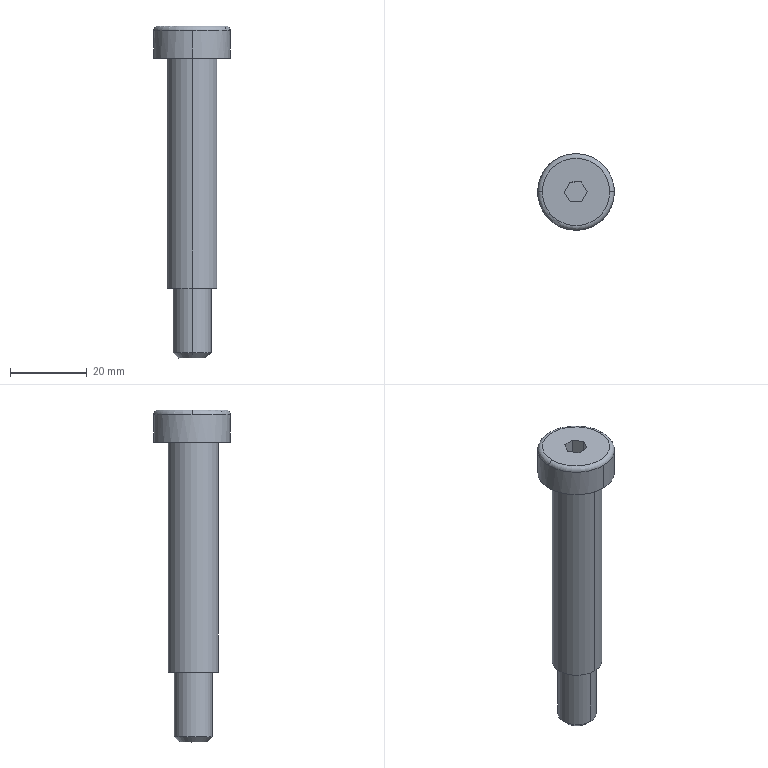Part | SolidWorks | features BaseBody 1 | 1 solid | 21 faces | box 20.001 x 20 x 86.624 mm | volume 11847 mm3 | plane 11 | cylinder 6 | torus 2 | cone 2 | commonest cylinder face diameters 10 x2 13 x2 20 x2
STEP:
#1=CARTESIAN_POINT('',(405.875,-5.722,120.785));
#2=VERTEX_POINT('',#1);
#3=CARTESIAN_POINT('',(396.085,-15.72,120.784));
#4=VERTEX_POINT('',#3);
#5=CARTESIAN_POINT('',(406.085,-15.72,120.785));
#6=DIRECTION('',(-0.0001435,-0.000000521,1.));
#7=DIRECTION('',(0.02104,-0.9998,0.000002497));
#8=AXIS2_PLACEMENT_3D('',#5,#6,#7);
#9=CIRCLE('',#8,10.);
#10=EDGE_CURVE('',#2,#4,#9,.T.);
#11=ORIENTED_EDGE('',*,*,#10,.T.);
#12=CARTESIAN_POINT('',(397.285,-15.72,121.984));
#13=VERTEX_POINT('',#12);
#14=CARTESIAN_POINT('',(397.285,-15.72,120.784));
#15=DIRECTION('',(0.,1.,0.000000521));
#16=DIRECTION('',(0.,-0.000000521,1.));
#17=AXIS2_PLACEMENT_3D('',#14,#15,#16);
#18=CIRCLE('',#17,1.2);
#19=EDGE_CURVE('',#4,#13,#18,.T.);
#20=ORIENTED_EDGE('',*,*,#19,.T.);
#21=CARTESIAN_POINT('',(414.885,-15.72,121.986));
#22=VERTEX_POINT('',#21);
#23=CARTESIAN_POINT('',(406.085,-15.72,121.985));
#24=DIRECTION('',(-0.0001435,-0.000000521,1.));
#25=DIRECTION('',(-1.,0.,-0.0001435));
#26=AXIS2_PLACEMENT_3D('',#23,#24,#25);
#27=CIRCLE('',#26,8.8);
#28=EDGE_CURVE('',#22,#13,#27,.T.);
#29=ORIENTED_EDGE('',*,*,#28,.F.);
#30=CARTESIAN_POINT('',(416.085,-15.72,120.786));
#31=VERTEX_POINT('',#30);
#32=CARTESIAN_POINT('',(414.885,-15.72,120.786));
#33=DIRECTION('',(0.,-1.,-0.000000521));
#34=DIRECTION('',(0.,0.000000521,-1.));
#35=AXIS2_PLACEMENT_3D('',#32,#33,#34);
#36=CIRCLE('',#35,1.2);
#37=EDGE_CURVE('',#31,#22,#36,.T.);
#38=ORIENTED_EDGE('',*,*,#37,.F.);
#39=CARTESIAN_POINT('',(406.085,-15.72,120.785));
#40=DIRECTION('',(-0.0001435,-0.000000521,1.));
#41=DIRECTION('',(0.02104,-0.9998,0.000002497));
#42=AXIS2_PLACEMENT_3D('',#39,#40,#41);
#43=CIRCLE('',#42,10.);
#44=EDGE_CURVE('',#31,#2,#43,.T.);
#45=ORIENTED_EDGE('',*,*,#44,.T.);
#46=EDGE_LOOP('',(#11,#20,#29,#38,#45));
#47=FACE_OUTER_BOUND('',#46,.T.);
#48=CARTESIAN_POINT('',(406.085,-15.72,120.785));
#49=DIRECTION('',(-0.0001435,-0.000000521,1.));
#50=DIRECTION('',(1.,0.,0.0001435));
#51=AXIS2_PLACEMENT_3D('',#48,#49,#50);
#52=TOROIDAL_SURFACE('',#51,8.8,1.2);
#53=ADVANCED_FACE('',(#47),#52,.T.);
#54=CARTESIAN_POINT('',(406.296,-25.717,113.585));
#55=VERTEX_POINT('',#54);
#56=CARTESIAN_POINT('',(405.876,-5.722,113.585));
#57=VERTEX_POINT('',#56);
#58=CARTESIAN_POINT('',(406.086,-15.72,113.585));
#59=DIRECTION('',(0.0001435,0.000000521,-1.));
#60=DIRECTION('',(-1.,0.,-0.0001435));
#61=AXIS2_PLACEMENT_3D('',#58,#59,#60);
#62=CIRCLE('',#61,10.);
#63=EDGE_CURVE('',#55,#57,#62,.T.);
#64=ORIENTED_EDGE('',*,*,#63,.F.);
#65=CARTESIAN_POINT('',(406.295,-25.717,120.785));
#66=VERTEX_POINT('',#65);
#67=CARTESIAN_POINT('',(406.296,-25.717,113.585));
#68=DIRECTION('',(-0.0001435,-0.000000521,1.));
#69=VECTOR('',#68,1000.);
#70=LINE('',#67,#69);
#71=EDGE_CURVE('',#55,#66,#70,.T.);
#72=ORIENTED_EDGE('',*,*,#71,.T.);
#73=CARTESIAN_POINT('',(406.085,-15.72,120.785));
#74=DIRECTION('',(-0.0001435,-0.000000521,1.));
#75=DIRECTION('',(0.02104,-0.9998,0.000002497));
#76=AXIS2_PLACEMENT_3D('',#73,#74,#75);
#77=CIRCLE('',#76,10.);
#78=EDGE_CURVE('',#4,#66,#77,.T.);
#79=ORIENTED_EDGE('',*,*,#78,.F.);
#80=ORIENTED_EDGE('',*,*,#10,.F.);
#81=CARTESIAN_POINT('',(405.876,-5.722,113.585));
#82=DIRECTION('',(-0.0001435,-0.000000521,1.));
#83=VECTOR('',#82,1000.);
#84=LINE('',#81,#83);
#85=EDGE_CURVE('',#57,#2,#84,.T.);
#86=ORIENTED_EDGE('',*,*,#85,.F.);
#87=EDGE_LOOP('',(#64,#72,#79,#80,#86));
#88=FACE_OUTER_BOUND('',#87,.T.);
#89=CARTESIAN_POINT('',(406.086,-15.72,113.585));
#90=DIRECTION('',(-0.0001435,-0.000000521,1.));
#91=DIRECTION('',(-0.02104,0.9998,-0.000002497));
#92=AXIS2_PLACEMENT_3D('',#89,#90,#91);
#93=CYLINDRICAL_SURFACE('',#92,10.);
#94=ADVANCED_FACE('',(#88),#93,.T.);
#95=CARTESIAN_POINT('',(405.959,-9.559,113.585));
#96=VERTEX_POINT('',#95);
#97=CARTESIAN_POINT('',(406.233,-22.556,113.585));
#98=VERTEX_POINT('',#97);
#99=CARTESIAN_POINT('',(406.096,-16.057,113.585));
#100=DIRECTION('',(-0.0001435,-0.000000521,1.));
#101=DIRECTION('',(0.02104,-0.9998,0.000002497));
#102=AXIS2_PLACEMENT_3D('',#99,#100,#101);
#103=CIRCLE('',#102,6.5);
#104=EDGE_CURVE('',#96,#98,#103,.T.);
#105=ORIENTED_EDGE('',*,*,#104,.F.);
#106=CARTESIAN_POINT('',(405.968,-9.558,53.585));
#107=VERTEX_POINT('',#106);
#108=CARTESIAN_POINT('',(405.964,-9.559,81.389));
#109=DIRECTION('',(0.0001435,0.000000521,-1.));
#110=VECTOR('',#109,1000.);
#111=LINE('',#108,#110);
#112=EDGE_CURVE('',#96,#107,#111,.T.);
#113=ORIENTED_EDGE('',*,*,#112,.T.);
#114=CARTESIAN_POINT('',(406.242,-22.556,53.585));
#115=VERTEX_POINT('',#114);
#116=CARTESIAN_POINT('',(406.105,-16.057,53.585));
#117=DIRECTION('',(0.0001435,0.000000521,-1.));
#118=DIRECTION('',(-1.,0.,-0.0001435));
#119=AXIS2_PLACEMENT_3D('',#116,#117,#118);
#120=CIRCLE('',#119,6.5);
#121=EDGE_CURVE('',#115,#107,#120,.T.);
#122=ORIENTED_EDGE('',*,*,#121,.F.);
#123=CARTESIAN_POINT('',(406.238,-22.556,81.389));
#124=DIRECTION('',(0.0001435,0.000000521,-1.));
#125=VECTOR('',#124,1000.);
#126=LINE('',#123,#125);
#127=EDGE_CURVE('',#98,#115,#126,.T.);
#128=ORIENTED_EDGE('',*,*,#127,.F.);
#129=EDGE_LOOP('',(#105,#113,#122,#128));
#130=FACE_OUTER_BOUND('',#129,.T.);
#131=CARTESIAN_POINT('',(406.101,-16.057,81.389));
#132=DIRECTION('',(0.0001435,0.000000521,-1.));
#133=DIRECTION('',(0.02104,-0.9998,0.000002497));
#134=AXIS2_PLACEMENT_3D('',#131,#132,#133);
#135=CYLINDRICAL_SURFACE('',#134,6.5);
#136=ADVANCED_FACE('',(#130),#135,.T.);
#137=CARTESIAN_POINT('',(405.998,-11.058,53.585));
#138=VERTEX_POINT('',#137);
#139=CARTESIAN_POINT('',(406.208,-21.056,53.585));
#140=VERTEX_POINT('',#139);
#141=CARTESIAN_POINT('',(406.103,-16.057,53.585));
#142=DIRECTION('',(-0.0001435,-0.000000521,1.));
#143=DIRECTION('',(0.02104,-0.9998,0.000002497));
#144=AXIS2_PLACEMENT_3D('',#141,#142,#143);
#145=CIRCLE('',#144,5.);
#146=EDGE_CURVE('',#138,#140,#145,.T.);
#147=ORIENTED_EDGE('',*,*,#146,.F.);
#148=CARTESIAN_POINT('',(406.,-11.058,36.763));
#149=VERTEX_POINT('',#148);
#150=CARTESIAN_POINT('',(405.999,-11.058,48.803));
#151=DIRECTION('',(0.0001435,0.000000521,-1.));
#152=VECTOR('',#151,1000.);
#153=LINE('',#150,#152);
#154=EDGE_CURVE('',#138,#149,#153,.T.);
#155=ORIENTED_EDGE('',*,*,#154,.T.);
#156=CARTESIAN_POINT('',(406.211,-21.056,36.763));
#157=VERTEX_POINT('',#156);
#158=CARTESIAN_POINT('',(406.106,-16.057,36.763));
#159=DIRECTION('',(0.0001435,0.000000521,-1.));
#160=DIRECTION('',(0.02104,-0.9998,0.000002497));
#161=AXIS2_PLACEMENT_3D('',#158,#159,#160);
#162=CIRCLE('',#161,5.);
#163=EDGE_CURVE('',#157,#149,#162,.T.);
#164=ORIENTED_EDGE('',*,*,#163,.F.);
#165=CARTESIAN_POINT('',(406.209,-21.056,48.803));
#166=DIRECTION('',(0.0001435,0.000000521,-1.));
#167=VECTOR('',#166,1000.);
#168=LINE('',#165,#167);
#169=EDGE_CURVE('',#140,#157,#168,.T.);
#170=ORIENTED_EDGE('',*,*,#169,.F.);
#171=EDGE_LOOP('',(#147,#155,#164,#170));
#172=FACE_OUTER_BOUND('',#171,.T.);
#173=CARTESIAN_POINT('',(406.104,-16.057,48.803));
#174=DIRECTION('',(0.0001435,0.000000521,-1.));
#175=DIRECTION('',(0.02104,-0.9998,0.000002497));
#176=AXIS2_PLACEMENT_3D('',#173,#174,#175);
#177=CYLINDRICAL_SURFACE('',#176,5.);
#178=ADVANCED_FACE('',(#172),#177,.T.);
#179=CARTESIAN_POINT('',(406.181,-19.656,35.363));
#180=VERTEX_POINT('',#179);
#181=CARTESIAN_POINT('',(406.03,-12.458,35.363));
#182=VERTEX_POINT('',#181);
#183=CARTESIAN_POINT('',(406.106,-16.057,35.363));
#184=DIRECTION('',(0.0001435,0.000000521,-1.));
#185=DIRECTION('',(0.02104,-0.9998,0.000002497));
#186=AXIS2_PLACEMENT_3D('',#183,#184,#185);
#187=CIRCLE('',#186,3.6);
#188=EDGE_CURVE('',#180,#182,#187,.T.);
#189=ORIENTED_EDGE('',*,*,#188,.F.);
#190=CARTESIAN_POINT('',(406.196,-20.356,36.063));
#191=DIRECTION('',(0.01477,-0.707,0.7071));
#192=VECTOR('',#191,1000.);
#193=LINE('',#190,#192);
#194=EDGE_CURVE('',#180,#157,#193,.T.);
#195=ORIENTED_EDGE('',*,*,#194,.T.);
#196=ORIENTED_EDGE('',*,*,#163,.T.);
#197=CARTESIAN_POINT('',(406.015,-11.758,36.063));
#198=DIRECTION('',(-0.01498,0.7069,0.7071));
#199=VECTOR('',#198,1000.);
#200=LINE('',#197,#199);
#201=EDGE_CURVE('',#182,#149,#200,.T.);
#202=ORIENTED_EDGE('',*,*,#201,.F.);
#203=EDGE_LOOP('',(#189,#195,#196,#202));
#204=FACE_OUTER_BOUND('',#203,.T.);
#205=CARTESIAN_POINT('',(406.106,-16.057,36.063));
#206=DIRECTION('',(-0.0001435,-0.000000521,1.));
#207=DIRECTION('',(-0.02104,0.9998,-0.000002497));
#208=AXIS2_PLACEMENT_3D('',#205,#206,#207);
#209=CONICAL_SURFACE('',#208,4.3,0.7854);
#210=ADVANCED_FACE('',(#204),#209,.T.);
#211=CARTESIAN_POINT('',(406.106,-16.057,35.363));
#212=DIRECTION('',(0.0001435,0.000000521,-1.));
#213=DIRECTION('',(0.02104,-0.9998,0.000002497));
#214=AXIS2_PLACEMENT_3D('',#211,#212,#213);
#215=CIRCLE('',#214,3.6);
#216=EDGE_CURVE('',#182,#180,#215,.T.);
#217=ORIENTED_EDGE('',*,*,#216,.T.);
#218=ORIENTED_EDGE('',*,*,#188,.T.);
#219=EDGE_LOOP('',(#217,#218));
#220=FACE_OUTER_BOUND('',#219,.T.);
#221=CARTESIAN_POINT('',(406.106,-16.057,35.363));
#222=DIRECTION('',(0.0001435,0.000000521,-1.));
#223=DIRECTION('',(0.,-1.,-0.000000521));
#224=AXIS2_PLACEMENT_3D('',#221,#222,#223);
#225=PLANE('',#224);
#226=ADVANCED_FACE('',(#220),#225,.T.);
#227=ORIENTED_EDGE('',*,*,#194,.F.);
#228=ORIENTED_EDGE('',*,*,#216,.F.);
#229=ORIENTED_EDGE('',*,*,#201,.T.);
#230=CARTESIAN_POINT('',(406.106,-16.057,36.763));
#231=DIRECTION('',(0.0001435,0.000000521,-1.));
#232=DIRECTION('',(0.02104,-0.9998,0.000002497));
#233=AXIS2_PLACEMENT_3D('',#230,#231,#232);
#234=CIRCLE('',#233,5.);
#235=EDGE_CURVE('',#149,#157,#234,.T.);
#236=ORIENTED_EDGE('',*,*,#235,.T.);
#237=EDGE_LOOP('',(#227,#228,#229,#236));
#238=FACE_OUTER_BOUND('',#237,.T.);
#239=CARTESIAN_POINT('',(406.106,-16.057,36.063));
#240=DIRECTION('',(-0.0001435,-0.000000521,1.));
#241=DIRECTION('',(-0.02104,0.9998,-0.000002497));
#242=AXIS2_PLACEMENT_3D('',#239,#240,#241);
#243=CONICAL_SURFACE('',#242,4.3,0.7854);
#244=ADVANCED_FACE('',(#238),#243,.T.);
#245=ORIENTED_EDGE('',*,*,#154,.F.);
#246=CARTESIAN_POINT('',(406.103,-16.057,53.585));
#247=DIRECTION('',(-0.0001435,-0.000000521,1.));
#248=DIRECTION('',(0.02104,-0.9998,0.000002497));
#249=AXIS2_PLACEMENT_3D('',#246,#247,#248);
#250=CIRCLE('',#249,5.);
#251=EDGE_CURVE('',#140,#138,#250,.T.);
#252=ORIENTED_EDGE('',*,*,#251,.F.);
#253=ORIENTED_EDGE('',*,*,#169,.T.);
#254=ORIENTED_EDGE('',*,*,#235,.F.);
#255=EDGE_LOOP('',(#245,#252,#253,#254));
#256=FACE_OUTER_BOUND('',#255,.T.);
#257=CARTESIAN_POINT('',(406.104,-16.057,48.803));
#258=DIRECTION('',(0.0001435,0.000000521,-1.));
#259=DIRECTION('',(0.02104,-0.9998,0.000002497));
#260=AXIS2_PLACEMENT_3D('',#257,#258,#259);
#261=CYLINDRICAL_SURFACE('',#260,5.);
#262=ADVANCED_FACE('',(#256),#261,.T.);
#263=ORIENTED_EDGE('',*,*,#251,.T.);
#264=ORIENTED_EDGE('',*,*,#146,.T.);
#265=EDGE_LOOP('',(#263,#264));
#266=FACE_BOUND('',#265,.T.);
#267=ORIENTED_EDGE('',*,*,#121,.T.);
#268=CARTESIAN_POINT('',(406.105,-16.057,53.585));
#269=DIRECTION('',(0.0001435,0.000000521,-1.));
#270=DIRECTION('',(-1.,0.,-0.0001435));
#271=AXIS2_PLACEMENT_3D('',#268,#269,#270);
#272=CIRCLE('',#271,6.5);
#273=EDGE_CURVE('',#107,#115,#272,.T.);
#274=ORIENTED_EDGE('',*,*,#273,.T.);
#275=EDGE_LOOP('',(#267,#274));
#276=FACE_OUTER_BOUND('',#275,.T.);
#277=CARTESIAN_POINT('',(406.09,-15.72,53.585));
#278=DIRECTION('',(0.0001435,0.000000521,-1.));
#279=DIRECTION('',(0.,-1.,-0.000000521));
#280=AXIS2_PLACEMENT_3D('',#277,#278,#279);
#281=PLANE('',#280);
#282=ADVANCED_FACE('',(#266,#276),#281,.T.);
#283=ORIENTED_EDGE('',*,*,#112,.F.);
#284=CARTESIAN_POINT('',(406.096,-16.057,113.585));
#285=DIRECTION('',(-0.0001435,-0.000000521,1.));
#286=DIRECTION('',(0.02104,-0.9998,0.000002497));
#287=AXIS2_PLACEMENT_3D('',#284,#285,#286);
#288=CIRCLE('',#287,6.5);
#289=EDGE_CURVE('',#98,#96,#288,.T.);
#290=ORIENTED_EDGE('',*,*,#289,.F.);
#291=ORIENTED_EDGE('',*,*,#127,.T.);
#292=ORIENTED_EDGE('',*,*,#273,.F.);
#293=EDGE_LOOP('',(#283,#290,#291,#292));
#294=FACE_OUTER_BOUND('',#293,.T.);
#295=CARTESIAN_POINT('',(406.101,-16.057,81.389));
#296=DIRECTION('',(0.0001435,0.000000521,-1.));
#297=DIRECTION('',(0.02104,-0.9998,0.000002497));
#298=AXIS2_PLACEMENT_3D('',#295,#296,#297);
#299=CYLINDRICAL_SURFACE('',#298,6.5);
#300=ADVANCED_FACE('',(#294),#299,.T.);
#301=ORIENTED_EDGE('',*,*,#289,.T.);
#302=ORIENTED_EDGE('',*,*,#104,.T.);
#303=EDGE_LOOP('',(#301,#302));
#304=FACE_BOUND('',#303,.T.);
#305=CARTESIAN_POINT('',(406.086,-15.72,113.585));
#306=DIRECTION('',(0.0001435,0.000000521,-1.));
#307=DIRECTION('',(-1.,0.,-0.0001435));
#308=AXIS2_PLACEMENT_3D('',#305,#306,#307);
#309=CIRCLE('',#308,10.);
#310=EDGE_CURVE('',#57,#55,#309,.T.);
#311=ORIENTED_EDGE('',*,*,#310,.T.);
#312=ORIENTED_EDGE('',*,*,#63,.T.);
#313=EDGE_LOOP('',(#311,#312));
#314=FACE_OUTER_BOUND('',#313,.T.);
#315=CARTESIAN_POINT('',(406.086,-15.72,113.585));
#316=DIRECTION('',(0.0001435,0.000000521,-1.));
#317=DIRECTION('',(0.,-1.,-0.000000521));
#318=AXIS2_PLACEMENT_3D('',#315,#316,#317);
#319=PLANE('',#318);
#320=ADVANCED_FACE('',(#304,#314),#319,.T.);
#321=ORIENTED_EDGE('',*,*,#71,.F.);
#322=ORIENTED_EDGE('',*,*,#310,.F.);
#323=ORIENTED_EDGE('',*,*,#85,.T.);
#324=ORIENTED_EDGE('',*,*,#44,.F.);
#325=CARTESIAN_POINT('',(406.085,-15.72,120.785));
#326=DIRECTION('',(-0.0001435,-0.000000521,1.));
#327=DIRECTION('',(0.02104,-0.9998,0.000002497));
#328=AXIS2_PLACEMENT_3D('',#325,#326,#327);
#329=CIRCLE('',#328,10.);
#330=EDGE_CURVE('',#66,#31,#329,.T.);
#331=ORIENTED_EDGE('',*,*,#330,.F.);
#332=EDGE_LOOP('',(#321,#322,#323,#324,#331));
#333=FACE_OUTER_BOUND('',#332,.T.);
#334=CARTESIAN_POINT('',(406.086,-15.72,113.585));
#335=DIRECTION('',(-0.0001435,-0.000000521,1.));
#336=DIRECTION('',(-0.02104,0.9998,-0.000002497));
#337=AXIS2_PLACEMENT_3D('',#334,#335,#336);
#338=CYLINDRICAL_SURFACE('',#337,10.);
#339=ADVANCED_FACE('',(#333),#338,.T.);
#340=ORIENTED_EDGE('',*,*,#19,.F.);
#341=ORIENTED_EDGE('',*,*,#78,.T.);
#342=ORIENTED_EDGE('',*,*,#330,.T.);
#343=ORIENTED_EDGE('',*,*,#37,.T.);
#344=CARTESIAN_POINT('',(406.085,-15.72,121.985));
#345=DIRECTION('',(-0.0001435,-0.000000521,1.));
#346=DIRECTION('',(-1.,0.,-0.0001435));
#347=AXIS2_PLACEMENT_3D('',#344,#345,#346);
#348=CIRCLE('',#347,8.8);
#349=EDGE_CURVE('',#13,#22,#348,.T.);
#350=ORIENTED_EDGE('',*,*,#349,.F.);
#351=EDGE_LOOP('',(#340,#341,#342,#343,#350));
#352=FACE_OUTER_BOUND('',#351,.T.);
#353=CARTESIAN_POINT('',(406.085,-15.72,120.785));
#354=DIRECTION('',(-0.0001435,-0.000000521,1.));
#355=DIRECTION('',(1.,0.,0.0001435));
#356=AXIS2_PLACEMENT_3D('',#353,#354,#355);
#357=TOROIDAL_SURFACE('',#356,8.8,1.2);
#358=ADVANCED_FACE('',(#352),#357,.T.);
#359=CARTESIAN_POINT('',(404.584,-18.33,115.985));
#360=VERTEX_POINT('',#359);
#361=CARTESIAN_POINT('',(407.583,-18.267,115.985));
#362=VERTEX_POINT('',#361);
#363=CARTESIAN_POINT('',(404.584,-18.33,115.985));
#364=DIRECTION('',(0.9998,0.02104,0.0001435));
#365=VECTOR('',#364,1000.);
#366=LINE('',#363,#365);
#367=EDGE_CURVE('',#360,#362,#366,.T.);
#368=ORIENTED_EDGE('',*,*,#367,.T.);
#369=CARTESIAN_POINT('',(409.028,-15.638,115.985));
#370=VERTEX_POINT('',#369);
#371=CARTESIAN_POINT('',(407.583,-18.267,115.985));
#372=DIRECTION('',(0.4817,0.8764,0.00006956));
#373=VECTOR('',#372,1000.);
#374=LINE('',#371,#373);
#375=EDGE_CURVE('',#362,#370,#374,.T.);
#376=ORIENTED_EDGE('',*,*,#375,.T.);
#377=CARTESIAN_POINT('',(407.474,-13.072,115.985));
#378=VERTEX_POINT('',#377);
#379=CARTESIAN_POINT('',(409.028,-15.638,115.985));
#380=DIRECTION('',(-0.5181,0.8553,-0.00007389));
#381=VECTOR('',#380,1000.);
#382=LINE('',#379,#381);
#383=EDGE_CURVE('',#370,#378,#382,.T.);
#384=ORIENTED_EDGE('',*,*,#383,.T.);
#385=CARTESIAN_POINT('',(404.474,-13.135,115.985));
#386=VERTEX_POINT('',#385);
#387=CARTESIAN_POINT('',(407.474,-13.072,115.985));
#388=DIRECTION('',(-0.9998,-0.02104,-0.0001435));
#389=VECTOR('',#388,1000.);
#390=LINE('',#387,#389);
#391=EDGE_CURVE('',#378,#386,#390,.T.);
#392=ORIENTED_EDGE('',*,*,#391,.T.);
#393=CARTESIAN_POINT('',(403.029,-15.764,115.985));
#394=VERTEX_POINT('',#393);
#395=CARTESIAN_POINT('',(404.474,-13.135,115.985));
#396=DIRECTION('',(-0.4817,-0.8764,-0.00006956));
#397=VECTOR('',#396,1000.);
#398=LINE('',#395,#397);
#399=EDGE_CURVE('',#386,#394,#398,.T.);
#400=ORIENTED_EDGE('',*,*,#399,.T.);
#401=CARTESIAN_POINT('',(403.029,-15.764,115.985));
#402=DIRECTION('',(0.5181,-0.8553,0.00007389));
#403=VECTOR('',#402,1000.);
#404=LINE('',#401,#403);
#405=EDGE_CURVE('',#394,#360,#404,.T.);
#406=ORIENTED_EDGE('',*,*,#405,.T.);
#407=EDGE_LOOP('',(#368,#376,#384,#392,#400,#406));
#408=FACE_OUTER_BOUND('',#407,.T.);
#409=CARTESIAN_POINT('',(405.473,13.374,115.985));
#410=DIRECTION('',(-0.0001435,-0.000000521,1.));
#411=DIRECTION('',(-0.003633,1.,0.));
#412=AXIS2_PLACEMENT_3D('',#409,#410,#411);
#413=PLANE('',#412);
#414=ADVANCED_FACE('',(#408),#413,.T.);
#415=CARTESIAN_POINT('',(407.582,-18.267,121.985));
#416=VERTEX_POINT('',#415);
#417=CARTESIAN_POINT('',(407.582,-18.267,121.985));
#418=DIRECTION('',(0.0001435,0.000000521,-1.));
#419=VECTOR('',#418,1000.);
#420=LINE('',#417,#419);
#421=EDGE_CURVE('',#416,#362,#420,.T.);
#422=ORIENTED_EDGE('',*,*,#421,.T.);
#423=ORIENTED_EDGE('',*,*,#367,.F.);
#424=CARTESIAN_POINT('',(404.583,-18.33,121.985));
#425=VERTEX_POINT('',#424);
#426=CARTESIAN_POINT('',(404.583,-18.33,121.985));
#427=DIRECTION('',(0.0001435,0.000000521,-1.));
#428=VECTOR('',#427,1000.);
#429=LINE('',#426,#428);
#430=EDGE_CURVE('',#425,#360,#429,.T.);
#431=ORIENTED_EDGE('',*,*,#430,.F.);
#432=CARTESIAN_POINT('',(407.582,-18.267,121.985));
#433=DIRECTION('',(-0.9998,-0.02104,-0.0001435));
#434=VECTOR('',#433,1000.);
#435=LINE('',#432,#434);
#436=EDGE_CURVE('',#416,#425,#435,.T.);
#437=ORIENTED_EDGE('',*,*,#436,.F.);
#438=EDGE_LOOP('',(#422,#423,#431,#437));
#439=FACE_OUTER_BOUND('',#438,.T.);
#440=CARTESIAN_POINT('',(407.583,-18.267,115.985));
#441=DIRECTION('',(0.02104,-0.9998,0.000002497));
#442=DIRECTION('',(0.,-0.000002498,-1.));
#443=AXIS2_PLACEMENT_3D('',#440,#441,#442);
#444=PLANE('',#443);
#445=ADVANCED_FACE('',(#439),#444,.F.);
#446=CARTESIAN_POINT('',(409.027,-15.638,121.985));
#447=VERTEX_POINT('',#446);
#448=CARTESIAN_POINT('',(409.027,-15.638,121.985));
#449=DIRECTION('',(0.0001435,0.000000521,-1.));
#450=VECTOR('',#449,1000.);
#451=LINE('',#448,#450);
#452=EDGE_CURVE('',#447,#370,#451,.T.);
#453=ORIENTED_EDGE('',*,*,#452,.T.);
#454=ORIENTED_EDGE('',*,*,#375,.F.);
#455=ORIENTED_EDGE('',*,*,#421,.F.);
#456=CARTESIAN_POINT('',(409.027,-15.638,121.985));
#457=DIRECTION('',(-0.4817,-0.8764,-0.00006956));
#458=VECTOR('',#457,1000.);
#459=LINE('',#456,#458);
#460=EDGE_CURVE('',#447,#416,#459,.T.);
#461=ORIENTED_EDGE('',*,*,#460,.F.);
#462=EDGE_LOOP('',(#453,#454,#455,#461));
#463=FACE_OUTER_BOUND('',#462,.T.);
#464=CARTESIAN_POINT('',(409.028,-15.638,115.985));
#465=DIRECTION('',(0.8764,-0.4817,0.0001255));
#466=DIRECTION('',(0.,-0.0002605,-1.));
#467=AXIS2_PLACEMENT_3D('',#464,#465,#466);
#468=PLANE('',#467);
#469=ADVANCED_FACE('',(#463),#468,.F.);
#470=CARTESIAN_POINT('',(407.473,-13.072,121.985));
#471=VERTEX_POINT('',#470);
#472=CARTESIAN_POINT('',(407.473,-13.072,121.985));
#473=DIRECTION('',(0.0001435,0.000000521,-1.));
#474=VECTOR('',#473,1000.);
#475=LINE('',#472,#474);
#476=EDGE_CURVE('',#471,#378,#475,.T.);
#477=ORIENTED_EDGE('',*,*,#476,.T.);
#478=ORIENTED_EDGE('',*,*,#383,.F.);
#479=ORIENTED_EDGE('',*,*,#452,.F.);
#480=CARTESIAN_POINT('',(407.473,-13.072,121.985));
#481=DIRECTION('',(0.5181,-0.8553,0.00007389));
#482=VECTOR('',#481,1000.);
#483=LINE('',#480,#482);
#484=EDGE_CURVE('',#471,#447,#483,.T.);
#485=ORIENTED_EDGE('',*,*,#484,.F.);
#486=EDGE_LOOP('',(#477,#478,#479,#485));
#487=FACE_OUTER_BOUND('',#486,.T.);
#488=CARTESIAN_POINT('',(407.474,-13.072,115.985));
#489=DIRECTION('',(0.8553,0.5181,0.000123));
#490=DIRECTION('',(0.,0.0002374,-1.));
#491=AXIS2_PLACEMENT_3D('',#488,#489,#490);
#492=PLANE('',#491);
#493=ADVANCED_FACE('',(#487),#492,.F.);
#494=CARTESIAN_POINT('',(404.473,-13.135,121.985));
#495=VERTEX_POINT('',#494);
#496=CARTESIAN_POINT('',(404.473,-13.135,121.985));
#497=DIRECTION('',(0.0001435,0.000000521,-1.));
#498=VECTOR('',#497,1000.);
#499=LINE('',#496,#498);
#500=EDGE_CURVE('',#495,#386,#499,.T.);
#501=ORIENTED_EDGE('',*,*,#500,.T.);
#502=ORIENTED_EDGE('',*,*,#391,.F.);
#503=ORIENTED_EDGE('',*,*,#476,.F.);
#504=CARTESIAN_POINT('',(404.473,-13.135,121.985));
#505=DIRECTION('',(0.9998,0.02104,0.0001435));
#506=VECTOR('',#505,1000.);
#507=LINE('',#504,#506);
#508=EDGE_CURVE('',#495,#471,#507,.T.);
#509=ORIENTED_EDGE('',*,*,#508,.F.);
#510=EDGE_LOOP('',(#501,#502,#503,#509));
#511=FACE_OUTER_BOUND('',#510,.T.);
#512=CARTESIAN_POINT('',(404.474,-13.135,115.985));
#513=DIRECTION('',(-0.02104,0.9998,-0.000002497));
#514=DIRECTION('',(-0.0001187,0.,1.));
#515=AXIS2_PLACEMENT_3D('',#512,#513,#514);
#516=PLANE('',#515);
#517=ADVANCED_FACE('',(#511),#516,.F.);
#518=CARTESIAN_POINT('',(403.028,-15.764,121.985));
#519=VERTEX_POINT('',#518);
#520=CARTESIAN_POINT('',(403.028,-15.764,121.985));
#521=DIRECTION('',(0.0001435,0.000000521,-1.));
#522=VECTOR('',#521,1000.);
#523=LINE('',#520,#522);
#524=EDGE_CURVE('',#519,#394,#523,.T.);
#525=ORIENTED_EDGE('',*,*,#524,.T.);
#526=ORIENTED_EDGE('',*,*,#399,.F.);
#527=ORIENTED_EDGE('',*,*,#500,.F.);
#528=CARTESIAN_POINT('',(403.028,-15.764,121.985));
#529=DIRECTION('',(0.4817,0.8764,0.00006956));
#530=VECTOR('',#529,1000.);
#531=LINE('',#528,#530);
#532=EDGE_CURVE('',#519,#495,#531,.T.);
#533=ORIENTED_EDGE('',*,*,#532,.F.);
#534=EDGE_LOOP('',(#525,#526,#527,#533));
#535=FACE_OUTER_BOUND('',#534,.T.);
#536=CARTESIAN_POINT('',(403.029,-15.764,115.985));
#537=DIRECTION('',(-0.8764,0.4817,-0.0001255));
#538=DIRECTION('',(-0.0001432,0.,1.));
#539=AXIS2_PLACEMENT_3D('',#536,#537,#538);
#540=PLANE('',#539);
#541=ADVANCED_FACE('',(#535),#540,.F.);
#542=ORIENTED_EDGE('',*,*,#430,.T.);
#543=ORIENTED_EDGE('',*,*,#405,.F.);
#544=ORIENTED_EDGE('',*,*,#524,.F.);
#545=CARTESIAN_POINT('',(404.583,-18.33,121.985));
#546=DIRECTION('',(-0.5181,0.8553,-0.00007389));
#547=VECTOR('',#546,1000.);
#548=LINE('',#545,#547);
#549=EDGE_CURVE('',#425,#519,#548,.T.);
#550=ORIENTED_EDGE('',*,*,#549,.F.);
#551=EDGE_LOOP('',(#542,#543,#544,#550));
#552=FACE_OUTER_BOUND('',#551,.T.);
#553=CARTESIAN_POINT('',(404.584,-18.33,115.985));
#554=DIRECTION('',(-0.8553,-0.5181,-0.000123));
#555=DIRECTION('',(-0.5181,0.8553,0.));
#556=AXIS2_PLACEMENT_3D('',#553,#554,#555);
#557=PLANE('',#556);
#558=ADVANCED_FACE('',(#552),#557,.F.);
#559=ORIENTED_EDGE('',*,*,#532,.T.);
#560=ORIENTED_EDGE('',*,*,#508,.T.);
#561=ORIENTED_EDGE('',*,*,#484,.T.);
#562=ORIENTED_EDGE('',*,*,#460,.T.);
#563=ORIENTED_EDGE('',*,*,#436,.T.);
#564=ORIENTED_EDGE('',*,*,#549,.T.);
#565=EDGE_LOOP('',(#559,#560,#561,#562,#563,#564));
#566=FACE_BOUND('',#565,.T.);
#567=ORIENTED_EDGE('',*,*,#28,.T.);
#568=ORIENTED_EDGE('',*,*,#349,.T.);
#569=EDGE_LOOP('',(#567,#568));
#570=FACE_OUTER_BOUND('',#569,.T.);
#571=CARTESIAN_POINT('',(406.085,-15.72,121.985));
#572=DIRECTION('',(-0.0001435,-0.000000521,1.));
#573=DIRECTION('',(-0.003633,1.,0.));
#574=AXIS2_PLACEMENT_3D('',#571,#572,#573);
#575=PLANE('',#574);
#576=ADVANCED_FACE('',(#566,#570),#575,.T.);
#577=CLOSED_SHELL('',(#53,#94,#136,#178,#210,#226,#244,#262,#282,#300,#320,#339,#358,#414,#445,#469,#493,#517,#541,#558,#576));
#578=MANIFOLD_SOLID_BREP('',#577);
#579=CARTESIAN_POINT('',(0.,0.,0.));
#580=DIRECTION('',(0.,0.,1.));
#581=DIRECTION('',(1.,0.,0.));
#582=AXIS2_PLACEMENT_3D('',#579,#580,#581);
#583=(LENGTH_UNIT()NAMED_UNIT(*)SI_UNIT(.MILLI.,.METRE.));
#584=UNCERTAINTY_MEASURE_WITH_UNIT(LENGTH_MEASURE(0.00001),#583,'','');
#585=(NAMED_UNIT(*)PLANE_ANGLE_UNIT()SI_UNIT($,.RADIAN.));
#586=(NAMED_UNIT(*)SI_UNIT($,.STERADIAN.)SOLID_ANGLE_UNIT());
#587=(GEOMETRIC_REPRESENTATION_CONTEXT(3)GLOBAL_UNCERTAINTY_ASSIGNED_CONTEXT((#584))GLOBAL_UNIT_ASSIGNED_CONTEXT((#583,#585,#586))REPRESENTATION_CONTEXT('',''));
#588=ADVANCED_BREP_SHAPE_REPRESENTATION('',(#578,#582),#587);